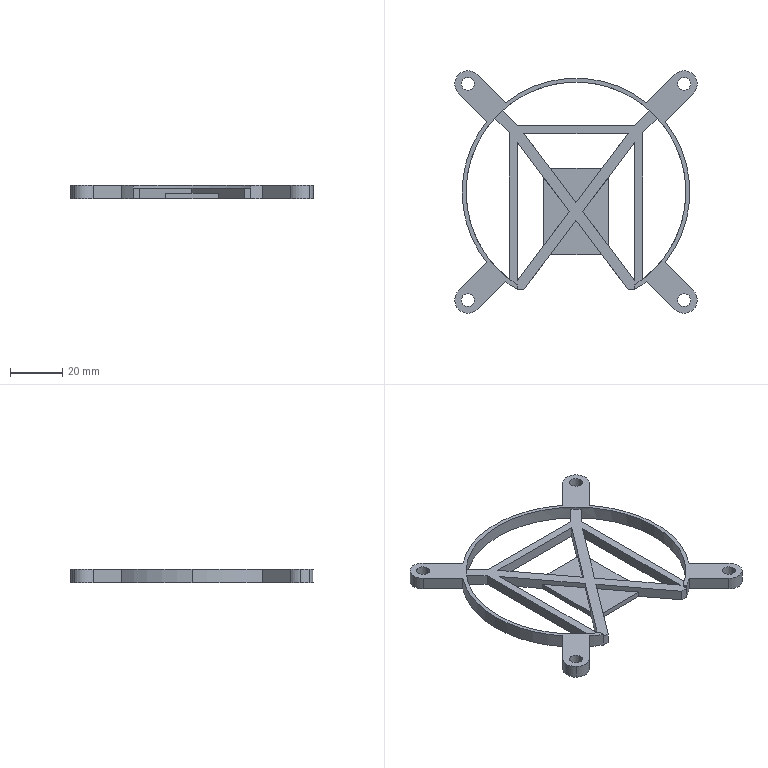Part | SolidWorks | features ICE 6, CirPattern 1, Extrusion 1, Fillet 1 | 1 solid | 68 faces | box 92.873 x 92.873 x 5 mm | volume 10601 mm3 | plane 41 | cylinder 27 | commonest cylinder face diameters 10 x10 5 x8 87.2 x6 84.2 x3